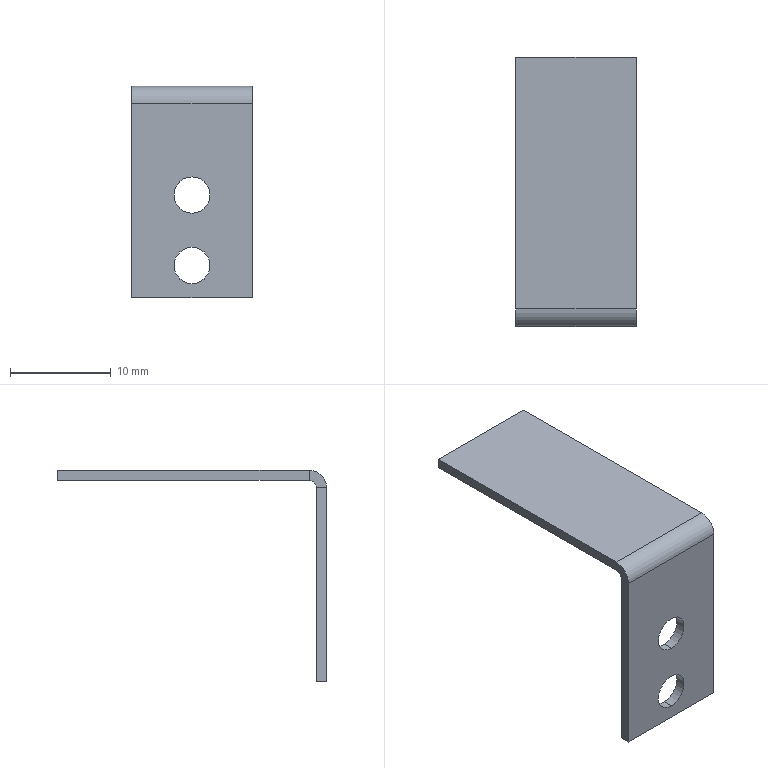Part | STEP file | PN_0031(Default) | 1 solid | 18 faces | box 12 x 26.737 x 21 mm | volume 534.113 mm3 | plane 12 | cylinder 6 | commonest cylinder face diameters 3.6 x4 1.473 x1 3.473 x1
STEP:
#1=CARTESIAN_POINT('',(0.,0.,0.));
#2=DIRECTION('',(0.,0.,1.));
#3=DIRECTION('',(1.,0.,0.));
#4=AXIS2_PLACEMENT_3D('',#1,#2,#3);
#5=CARTESIAN_POINT('',(0.,-0.7366,-12.6));
#6=VERTEX_POINT('',#5);
#7=CARTESIAN_POINT('',(0.,-1.737,-12.6));
#8=VERTEX_POINT('',#7);
#9=CARTESIAN_POINT('',(0.,-1.737,-12.6));
#10=DIRECTION('',(0.,-1.,0.));
#11=VECTOR('',#10,1.);
#12=LINE('',#9,#11);
#13=CARTESIAN_POINT('',(0.,-1.737,-10.8));
#14=DIRECTION('',(0.,-1.,0.));
#15=DIRECTION('',(0.,0.,-1.));
#16=AXIS2_PLACEMENT_3D('',#13,#14,#15);
#17=CYLINDRICAL_SURFACE('',#16,1.8);
#18=CARTESIAN_POINT('',(6.283,0.));
#19=DIRECTION('',(0.,1.));
#20=VECTOR('',#19,1.);
#21=LINE('',#18,#20);
#22=(GEOMETRIC_REPRESENTATION_CONTEXT(2)PARAMETRIC_REPRESENTATION_CONTEXT()REPRESENTATION_CONTEXT('',''));
#23=DEFINITIONAL_REPRESENTATION('',(#21),#22);
#24=PCURVE('',#17,#23);
#25=CARTESIAN_POINT('',(0.,-1.737,-10.8));
#26=DIRECTION('',(0.,-1.,0.));
#27=DIRECTION('',(0.,0.,-1.));
#28=AXIS2_PLACEMENT_3D('',#25,#26,#27);
#29=CYLINDRICAL_SURFACE('',#28,1.8);
#30=CARTESIAN_POINT('',(0.,0.));
#31=DIRECTION('',(0.,1.));
#32=VECTOR('',#31,1.);
#33=LINE('',#30,#32);
#34=(GEOMETRIC_REPRESENTATION_CONTEXT(2)PARAMETRIC_REPRESENTATION_CONTEXT()REPRESENTATION_CONTEXT('',''));
#35=DEFINITIONAL_REPRESENTATION('',(#33),#34);
#36=PCURVE('',#29,#35);
#37=SURFACE_CURVE('',#12,(#24,#36),.PCURVE_S1.);
#38=EDGE_CURVE('',#6,#8,#37,.T.);
#39=ORIENTED_EDGE('',*,*,#38,.T.);
#40=CARTESIAN_POINT('',(0.,-1.737,-9.));
#41=VERTEX_POINT('',#40);
#42=CARTESIAN_POINT('',(0.,-1.737,-10.8));
#43=DIRECTION('',(0.,-1.,0.));
#44=DIRECTION('',(0.,0.,-1.));
#45=AXIS2_PLACEMENT_3D('',#42,#43,#44);
#46=CIRCLE('',#45,1.8);
#47=CARTESIAN_POINT('',(0.,0.));
#48=DIRECTION('',(1.,0.));
#49=VECTOR('',#48,1.);
#50=LINE('',#47,#49);
#51=(GEOMETRIC_REPRESENTATION_CONTEXT(2)PARAMETRIC_REPRESENTATION_CONTEXT()REPRESENTATION_CONTEXT('',''));
#52=DEFINITIONAL_REPRESENTATION('',(#50),#51);
#53=PCURVE('',#17,#52);
#54=CARTESIAN_POINT('',(0.,-1.737,0.));
#55=DIRECTION('',(0.,1.,0.));
#56=DIRECTION('',(0.,0.,1.));
#57=AXIS2_PLACEMENT_3D('',#54,#55,#56);
#58=PLANE('',#57);
#59=CARTESIAN_POINT('',(-12.6,0.));
#60=CARTESIAN_POINT('',(-12.6,3.118));
#61=CARTESIAN_POINT('',(-9.9,1.559));
#62=CARTESIAN_POINT('',(-7.2,0.));
#63=CARTESIAN_POINT('',(-9.9,-1.559));
#64=CARTESIAN_POINT('',(-12.6,-3.118));
#65=CARTESIAN_POINT('',(-12.6,0.));
#66=(BOUNDED_CURVE()B_SPLINE_CURVE(2,(#59,#60,#61,#62,#63,#64,#65),.UNSPECIFIED.,.T.,.F.)B_SPLINE_CURVE_WITH_KNOTS((1,2,2,2,2,1),(-2.094,0.,2.094,4.189,6.283,8.378),.UNSPECIFIED.)CURVE()GEOMETRIC_REPRESENTATION_ITEM()RATIONAL_B_SPLINE_CURVE((1.,0.5,1.,0.5,1.,0.5,1.))REPRESENTATION_ITEM(''));
#67=(GEOMETRIC_REPRESENTATION_CONTEXT(2)PARAMETRIC_REPRESENTATION_CONTEXT()REPRESENTATION_CONTEXT('',''));
#68=DEFINITIONAL_REPRESENTATION('',(#66),#67);
#69=PCURVE('',#58,#68);
#70=SURFACE_CURVE('',#46,(#53,#69),.PCURVE_S1.);
#71=EDGE_CURVE('',#41,#8,#70,.T.);
#72=ORIENTED_EDGE('',*,*,#71,.F.);
#73=CARTESIAN_POINT('',(0.,-0.7366,-9.));
#74=VERTEX_POINT('',#73);
#75=CARTESIAN_POINT('',(0.,-1.737,-9.));
#76=DIRECTION('',(0.,-1.,0.));
#77=VECTOR('',#76,1.);
#78=LINE('',#75,#77);
#79=CARTESIAN_POINT('',(3.142,0.));
#80=DIRECTION('',(0.,1.));
#81=VECTOR('',#80,1.);
#82=LINE('',#79,#81);
#83=(GEOMETRIC_REPRESENTATION_CONTEXT(2)PARAMETRIC_REPRESENTATION_CONTEXT()REPRESENTATION_CONTEXT('',''));
#84=DEFINITIONAL_REPRESENTATION('',(#82),#83);
#85=PCURVE('',#17,#84);
#86=CARTESIAN_POINT('',(3.142,0.));
#87=DIRECTION('',(0.,1.));
#88=VECTOR('',#87,1.);
#89=LINE('',#86,#88);
#90=(GEOMETRIC_REPRESENTATION_CONTEXT(2)PARAMETRIC_REPRESENTATION_CONTEXT()REPRESENTATION_CONTEXT('',''));
#91=DEFINITIONAL_REPRESENTATION('',(#89),#90);
#92=PCURVE('',#29,#91);
#93=SURFACE_CURVE('',#78,(#85,#92),.PCURVE_S1.);
#94=EDGE_CURVE('',#74,#41,#93,.T.);
#95=ORIENTED_EDGE('',*,*,#94,.F.);
#96=CARTESIAN_POINT('',(0.,-0.7366,-10.8));
#97=DIRECTION('',(0.,1.,0.));
#98=DIRECTION('',(0.,0.,1.));
#99=AXIS2_PLACEMENT_3D('',#96,#97,#98);
#100=CIRCLE('',#99,1.8);
#101=CARTESIAN_POINT('',(9.425,-1.));
#102=DIRECTION('',(-1.,0.));
#103=VECTOR('',#102,1.);
#104=LINE('',#101,#103);
#105=(GEOMETRIC_REPRESENTATION_CONTEXT(2)PARAMETRIC_REPRESENTATION_CONTEXT()REPRESENTATION_CONTEXT('',''));
#106=DEFINITIONAL_REPRESENTATION('',(#104),#105);
#107=PCURVE('',#17,#106);
#108=CARTESIAN_POINT('',(0.,-0.7366,0.));
#109=DIRECTION('',(0.,1.,0.));
#110=DIRECTION('',(0.,0.,1.));
#111=AXIS2_PLACEMENT_3D('',#108,#109,#110);
#112=PLANE('',#111);
#113=CARTESIAN_POINT('',(-10.8,0.));
#114=DIRECTION('',(1.,0.));
#115=AXIS2_PLACEMENT_2D('',#113,#114);
#116=CIRCLE('',#115,1.8);
#117=(GEOMETRIC_REPRESENTATION_CONTEXT(2)PARAMETRIC_REPRESENTATION_CONTEXT()REPRESENTATION_CONTEXT('',''));
#118=DEFINITIONAL_REPRESENTATION('',(#116),#117);
#119=PCURVE('',#112,#118);
#120=SURFACE_CURVE('',#100,(#107,#119),.PCURVE_S1.);
#121=EDGE_CURVE('',#6,#74,#120,.T.);
#122=ORIENTED_EDGE('',*,*,#121,.F.);
#123=EDGE_LOOP('',(#39,#72,#95,#122));
#124=FACE_BOUND('',#123,.F.);
#125=ADVANCED_FACE('',(#124),#17,.F.);
#126=CARTESIAN_POINT('',(0.,-0.7366,-19.6));
#127=VERTEX_POINT('',#126);
#128=CARTESIAN_POINT('',(0.,-1.737,-19.6));
#129=VERTEX_POINT('',#128);
#130=CARTESIAN_POINT('',(0.,-1.737,-19.6));
#131=DIRECTION('',(0.,-1.,0.));
#132=VECTOR('',#131,1.);
#133=LINE('',#130,#132);
#134=CARTESIAN_POINT('',(0.,-1.737,-17.8));
#135=DIRECTION('',(0.,-1.,0.));
#136=DIRECTION('',(0.,0.,-1.));
#137=AXIS2_PLACEMENT_3D('',#134,#135,#136);
#138=CYLINDRICAL_SURFACE('',#137,1.8);
#139=CARTESIAN_POINT('',(6.283,0.));
#140=DIRECTION('',(0.,1.));
#141=VECTOR('',#140,1.);
#142=LINE('',#139,#141);
#143=(GEOMETRIC_REPRESENTATION_CONTEXT(2)PARAMETRIC_REPRESENTATION_CONTEXT()REPRESENTATION_CONTEXT('',''));
#144=DEFINITIONAL_REPRESENTATION('',(#142),#143);
#145=PCURVE('',#138,#144);
#146=CARTESIAN_POINT('',(0.,-1.737,-17.8));
#147=DIRECTION('',(0.,-1.,0.));
#148=DIRECTION('',(0.,0.,-1.));
#149=AXIS2_PLACEMENT_3D('',#146,#147,#148);
#150=CYLINDRICAL_SURFACE('',#149,1.8);
#151=CARTESIAN_POINT('',(0.,0.));
#152=DIRECTION('',(0.,1.));
#153=VECTOR('',#152,1.);
#154=LINE('',#151,#153);
#155=(GEOMETRIC_REPRESENTATION_CONTEXT(2)PARAMETRIC_REPRESENTATION_CONTEXT()REPRESENTATION_CONTEXT('',''));
#156=DEFINITIONAL_REPRESENTATION('',(#154),#155);
#157=PCURVE('',#150,#156);
#158=SURFACE_CURVE('',#133,(#145,#157),.PCURVE_S1.);
#159=EDGE_CURVE('',#127,#129,#158,.T.);
#160=ORIENTED_EDGE('',*,*,#159,.T.);
#161=CARTESIAN_POINT('',(0.,-1.737,-16.));
#162=VERTEX_POINT('',#161);
#163=CARTESIAN_POINT('',(0.,-1.737,-17.8));
#164=DIRECTION('',(0.,-1.,0.));
#165=DIRECTION('',(0.,0.,-1.));
#166=AXIS2_PLACEMENT_3D('',#163,#164,#165);
#167=CIRCLE('',#166,1.8);
#168=CARTESIAN_POINT('',(0.,0.));
#169=DIRECTION('',(1.,0.));
#170=VECTOR('',#169,1.);
#171=LINE('',#168,#170);
#172=(GEOMETRIC_REPRESENTATION_CONTEXT(2)PARAMETRIC_REPRESENTATION_CONTEXT()REPRESENTATION_CONTEXT('',''));
#173=DEFINITIONAL_REPRESENTATION('',(#171),#172);
#174=PCURVE('',#138,#173);
#175=CARTESIAN_POINT('',(-19.6,0.));
#176=CARTESIAN_POINT('',(-19.6,3.118));
#177=CARTESIAN_POINT('',(-16.9,1.559));
#178=CARTESIAN_POINT('',(-14.2,0.));
#179=CARTESIAN_POINT('',(-16.9,-1.559));
#180=CARTESIAN_POINT('',(-19.6,-3.118));
#181=CARTESIAN_POINT('',(-19.6,0.));
#182=(BOUNDED_CURVE()B_SPLINE_CURVE(2,(#175,#176,#177,#178,#179,#180,#181),.UNSPECIFIED.,.T.,.F.)B_SPLINE_CURVE_WITH_KNOTS((1,2,2,2,2,1),(-2.094,0.,2.094,4.189,6.283,8.378),.UNSPECIFIED.)CURVE()GEOMETRIC_REPRESENTATION_ITEM()RATIONAL_B_SPLINE_CURVE((1.,0.5,1.,0.5,1.,0.5,1.))REPRESENTATION_ITEM(''));
#183=(GEOMETRIC_REPRESENTATION_CONTEXT(2)PARAMETRIC_REPRESENTATION_CONTEXT()REPRESENTATION_CONTEXT('',''));
#184=DEFINITIONAL_REPRESENTATION('',(#182),#183);
#185=PCURVE('',#58,#184);
#186=SURFACE_CURVE('',#167,(#174,#185),.PCURVE_S1.);
#187=EDGE_CURVE('',#162,#129,#186,.T.);
#188=ORIENTED_EDGE('',*,*,#187,.F.);
#189=CARTESIAN_POINT('',(0.,-0.7366,-16.));
#190=VERTEX_POINT('',#189);
#191=CARTESIAN_POINT('',(0.,-1.737,-16.));
#192=DIRECTION('',(0.,-1.,0.));
#193=VECTOR('',#192,1.);
#194=LINE('',#191,#193);
#195=CARTESIAN_POINT('',(3.142,0.));
#196=DIRECTION('',(0.,1.));
#197=VECTOR('',#196,1.);
#198=LINE('',#195,#197);
#199=(GEOMETRIC_REPRESENTATION_CONTEXT(2)PARAMETRIC_REPRESENTATION_CONTEXT()REPRESENTATION_CONTEXT('',''));
#200=DEFINITIONAL_REPRESENTATION('',(#198),#199);
#201=PCURVE('',#138,#200);
#202=CARTESIAN_POINT('',(3.142,0.));
#203=DIRECTION('',(0.,1.));
#204=VECTOR('',#203,1.);
#205=LINE('',#202,#204);
#206=(GEOMETRIC_REPRESENTATION_CONTEXT(2)PARAMETRIC_REPRESENTATION_CONTEXT()REPRESENTATION_CONTEXT('',''));
#207=DEFINITIONAL_REPRESENTATION('',(#205),#206);
#208=PCURVE('',#150,#207);
#209=SURFACE_CURVE('',#194,(#201,#208),.PCURVE_S1.);
#210=EDGE_CURVE('',#190,#162,#209,.T.);
#211=ORIENTED_EDGE('',*,*,#210,.F.);
#212=CARTESIAN_POINT('',(0.,-0.7366,-17.8));
#213=DIRECTION('',(0.,1.,0.));
#214=DIRECTION('',(0.,0.,1.));
#215=AXIS2_PLACEMENT_3D('',#212,#213,#214);
#216=CIRCLE('',#215,1.8);
#217=CARTESIAN_POINT('',(9.425,-1.));
#218=DIRECTION('',(-1.,0.));
#219=VECTOR('',#218,1.);
#220=LINE('',#217,#219);
#221=(GEOMETRIC_REPRESENTATION_CONTEXT(2)PARAMETRIC_REPRESENTATION_CONTEXT()REPRESENTATION_CONTEXT('',''));
#222=DEFINITIONAL_REPRESENTATION('',(#220),#221);
#223=PCURVE('',#138,#222);
#224=CARTESIAN_POINT('',(-17.8,0.));
#225=DIRECTION('',(1.,0.));
#226=AXIS2_PLACEMENT_2D('',#224,#225);
#227=CIRCLE('',#226,1.8);
#228=(GEOMETRIC_REPRESENTATION_CONTEXT(2)PARAMETRIC_REPRESENTATION_CONTEXT()REPRESENTATION_CONTEXT('',''));
#229=DEFINITIONAL_REPRESENTATION('',(#227),#228);
#230=PCURVE('',#112,#229);
#231=SURFACE_CURVE('',#216,(#223,#230),.PCURVE_S1.);
#232=EDGE_CURVE('',#127,#190,#231,.T.);
#233=ORIENTED_EDGE('',*,*,#232,.F.);
#234=EDGE_LOOP('',(#160,#188,#211,#233));
#235=FACE_BOUND('',#234,.F.);
#236=ADVANCED_FACE('',(#235),#138,.F.);
#237=CARTESIAN_POINT('',(-6.,25.,0.));
#238=VERTEX_POINT('',#237);
#239=CARTESIAN_POINT('',(-6.,0.,0.));
#240=VERTEX_POINT('',#239);
#241=CARTESIAN_POINT('',(-6.,25.,0.));
#242=DIRECTION('',(0.,-1.,0.));
#243=VECTOR('',#242,1.);
#244=LINE('',#241,#243);
#245=CARTESIAN_POINT('',(-6.,25.,-1.));
#246=DIRECTION('',(-1.,0.,0.));
#247=DIRECTION('',(0.,-1.,0.));
#248=AXIS2_PLACEMENT_3D('',#245,#246,#247);
#249=PLANE('',#248);
#250=CARTESIAN_POINT('',(0.,1.));
#251=DIRECTION('',(1.,0.));
#252=VECTOR('',#251,1.);
#253=LINE('',#250,#252);
#254=(GEOMETRIC_REPRESENTATION_CONTEXT(2)PARAMETRIC_REPRESENTATION_CONTEXT()REPRESENTATION_CONTEXT('',''));
#255=DEFINITIONAL_REPRESENTATION('',(#253),#254);
#256=PCURVE('',#249,#255);
#257=CARTESIAN_POINT('',(0.,0.,0.));
#258=DIRECTION('',(0.,0.,1.));
#259=DIRECTION('',(1.,0.,0.));
#260=AXIS2_PLACEMENT_3D('',#257,#258,#259);
#261=PLANE('',#260);
#262=CARTESIAN_POINT('',(-6.,25.));
#263=DIRECTION('',(0.,-1.));
#264=VECTOR('',#263,1.);
#265=LINE('',#262,#264);
#266=(GEOMETRIC_REPRESENTATION_CONTEXT(2)PARAMETRIC_REPRESENTATION_CONTEXT()REPRESENTATION_CONTEXT('',''));
#267=DEFINITIONAL_REPRESENTATION('',(#265),#266);
#268=PCURVE('',#261,#267);
#269=SURFACE_CURVE('',#244,(#256,#268),.PCURVE_S1.);
#270=EDGE_CURVE('',#238,#240,#269,.T.);
#271=ORIENTED_EDGE('',*,*,#270,.F.);
#272=CARTESIAN_POINT('',(-6.,25.,-1.));
#273=VERTEX_POINT('',#272);
#274=CARTESIAN_POINT('',(-6.,25.,-1.));
#275=DIRECTION('',(0.,0.,1.));
#276=VECTOR('',#275,1.);
#277=LINE('',#274,#276);
#278=CARTESIAN_POINT('',(0.,0.));
#279=DIRECTION('',(0.,1.));
#280=VECTOR('',#279,1.);
#281=LINE('',#278,#280);
#282=(GEOMETRIC_REPRESENTATION_CONTEXT(2)PARAMETRIC_REPRESENTATION_CONTEXT()REPRESENTATION_CONTEXT('',''));
#283=DEFINITIONAL_REPRESENTATION('',(#281),#282);
#284=PCURVE('',#249,#283);
#285=CARTESIAN_POINT('',(-6.,25.,-1.));
#286=DIRECTION('',(0.,1.,0.));
#287=DIRECTION('',(0.,0.,1.));
#288=AXIS2_PLACEMENT_3D('',#285,#286,#287);
#289=PLANE('',#288);
#290=CARTESIAN_POINT('',(0.,0.));
#291=DIRECTION('',(1.,0.));
#292=VECTOR('',#291,1.);
#293=LINE('',#290,#292);
#294=(GEOMETRIC_REPRESENTATION_CONTEXT(2)PARAMETRIC_REPRESENTATION_CONTEXT()REPRESENTATION_CONTEXT('',''));
#295=DEFINITIONAL_REPRESENTATION('',(#293),#294);
#296=PCURVE('',#289,#295);
#297=SURFACE_CURVE('',#277,(#284,#296),.PCURVE_S1.);
#298=EDGE_CURVE('',#273,#238,#297,.T.);
#299=ORIENTED_EDGE('',*,*,#298,.F.);
#300=CARTESIAN_POINT('',(-6.,0.,-1.));
#301=VERTEX_POINT('',#300);
#302=CARTESIAN_POINT('',(-6.,25.,-1.));
#303=DIRECTION('',(0.,-1.,0.));
#304=VECTOR('',#303,1.);
#305=LINE('',#302,#304);
#306=CARTESIAN_POINT('',(0.,0.));
#307=DIRECTION('',(1.,0.));
#308=VECTOR('',#307,1.);
#309=LINE('',#306,#308);
#310=(GEOMETRIC_REPRESENTATION_CONTEXT(2)PARAMETRIC_REPRESENTATION_CONTEXT()REPRESENTATION_CONTEXT('',''));
#311=DEFINITIONAL_REPRESENTATION('',(#309),#310);
#312=PCURVE('',#249,#311);
#313=CARTESIAN_POINT('',(0.,0.,-1.));
#314=DIRECTION('',(0.,0.,1.));
#315=DIRECTION('',(1.,0.,0.));
#316=AXIS2_PLACEMENT_3D('',#313,#314,#315);
#317=PLANE('',#316);
#318=CARTESIAN_POINT('',(-6.,25.));
#319=DIRECTION('',(0.,-1.));
#320=VECTOR('',#319,1.);
#321=LINE('',#318,#320);
#322=(GEOMETRIC_REPRESENTATION_CONTEXT(2)PARAMETRIC_REPRESENTATION_CONTEXT()REPRESENTATION_CONTEXT('',''));
#323=DEFINITIONAL_REPRESENTATION('',(#321),#322);
#324=PCURVE('',#317,#323);
#325=SURFACE_CURVE('',#305,(#312,#324),.PCURVE_S1.);
#326=EDGE_CURVE('',#273,#301,#325,.T.);
#327=ORIENTED_EDGE('',*,*,#326,.T.);
#328=CARTESIAN_POINT('',(-6.,0.,-1.));
#329=DIRECTION('',(0.,0.,1.));
#330=VECTOR('',#329,1.);
#331=LINE('',#328,#330);
#332=CARTESIAN_POINT('',(25.,0.));
#333=DIRECTION('',(0.,1.));
#334=VECTOR('',#333,1.);
#335=LINE('',#332,#334);
#336=(GEOMETRIC_REPRESENTATION_CONTEXT(2)PARAMETRIC_REPRESENTATION_CONTEXT()REPRESENTATION_CONTEXT('',''));
#337=DEFINITIONAL_REPRESENTATION('',(#335),#336);
#338=PCURVE('',#249,#337);
#339=CARTESIAN_POINT('',(-6.,0.,-1.737));
#340=DIRECTION('',(1.,0.,0.));
#341=DIRECTION('',(0.,1.,0.));
#342=AXIS2_PLACEMENT_3D('',#339,#340,#341);
#343=PLANE('',#342);
#344=CARTESIAN_POINT('',(0.,0.7366));
#345=DIRECTION('',(0.,1.));
#346=VECTOR('',#345,1.);
#347=LINE('',#344,#346);
#348=(GEOMETRIC_REPRESENTATION_CONTEXT(2)PARAMETRIC_REPRESENTATION_CONTEXT()REPRESENTATION_CONTEXT('',''));
#349=DEFINITIONAL_REPRESENTATION('',(#347),#348);
#350=PCURVE('',#343,#349);
#351=SURFACE_CURVE('',#331,(#338,#350),.PCURVE_S1.);
#352=EDGE_CURVE('',#301,#240,#351,.T.);
#353=ORIENTED_EDGE('',*,*,#352,.T.);
#354=EDGE_LOOP('',(#271,#299,#327,#353));
#355=FACE_BOUND('',#354,.T.);
#356=ADVANCED_FACE('',(#355),#249,.T.);
#357=CARTESIAN_POINT('',(6.,25.,0.));
#358=VERTEX_POINT('',#357);
#359=CARTESIAN_POINT('',(-6.,25.,0.));
#360=DIRECTION('',(-1.,0.,0.));
#361=VECTOR('',#360,1.);
#362=LINE('',#359,#361);
#363=CARTESIAN_POINT('',(1.,0.));
#364=DIRECTION('',(0.,-1.));
#365=VECTOR('',#364,1.);
#366=LINE('',#363,#365);
#367=(GEOMETRIC_REPRESENTATION_CONTEXT(2)PARAMETRIC_REPRESENTATION_CONTEXT()REPRESENTATION_CONTEXT('',''));
#368=DEFINITIONAL_REPRESENTATION('',(#366),#367);
#369=PCURVE('',#289,#368);
#370=CARTESIAN_POINT('',(-6.,25.));
#371=DIRECTION('',(-1.,0.));
#372=VECTOR('',#371,1.);
#373=LINE('',#370,#372);
#374=(GEOMETRIC_REPRESENTATION_CONTEXT(2)PARAMETRIC_REPRESENTATION_CONTEXT()REPRESENTATION_CONTEXT('',''));
#375=DEFINITIONAL_REPRESENTATION('',(#373),#374);
#376=PCURVE('',#261,#375);
#377=SURFACE_CURVE('',#362,(#369,#376),.PCURVE_S1.);
#378=EDGE_CURVE('',#358,#238,#377,.T.);
#379=ORIENTED_EDGE('',*,*,#378,.F.);
#380=CARTESIAN_POINT('',(6.,25.,-1.));
#381=VERTEX_POINT('',#380);
#382=CARTESIAN_POINT('',(6.,25.,-1.));
#383=DIRECTION('',(0.,0.,1.));
#384=VECTOR('',#383,1.);
#385=LINE('',#382,#384);
#386=CARTESIAN_POINT('',(0.,12.));
#387=DIRECTION('',(1.,0.));
#388=VECTOR('',#387,1.);
#389=LINE('',#386,#388);
#390=(GEOMETRIC_REPRESENTATION_CONTEXT(2)PARAMETRIC_REPRESENTATION_CONTEXT()REPRESENTATION_CONTEXT('',''));
#391=DEFINITIONAL_REPRESENTATION('',(#389),#390);
#392=PCURVE('',#289,#391);
#393=CARTESIAN_POINT('',(6.,25.,-1.));
#394=DIRECTION('',(1.,0.,0.));
#395=DIRECTION('',(0.,1.,0.));
#396=AXIS2_PLACEMENT_3D('',#393,#394,#395);
#397=PLANE('',#396);
#398=CARTESIAN_POINT('',(0.,0.));
#399=DIRECTION('',(0.,1.));
#400=VECTOR('',#399,1.);
#401=LINE('',#398,#400);
#402=(GEOMETRIC_REPRESENTATION_CONTEXT(2)PARAMETRIC_REPRESENTATION_CONTEXT()REPRESENTATION_CONTEXT('',''));
#403=DEFINITIONAL_REPRESENTATION('',(#401),#402);
#404=PCURVE('',#397,#403);
#405=SURFACE_CURVE('',#385,(#392,#404),.PCURVE_S1.);
#406=EDGE_CURVE('',#381,#358,#405,.T.);
#407=ORIENTED_EDGE('',*,*,#406,.F.);
#408=CARTESIAN_POINT('',(-6.,25.,-1.));
#409=DIRECTION('',(-1.,0.,0.));
#410=VECTOR('',#409,1.);
#411=LINE('',#408,#410);
#412=CARTESIAN_POINT('',(0.,0.));
#413=DIRECTION('',(0.,-1.));
#414=VECTOR('',#413,1.);
#415=LINE('',#412,#414);
#416=(GEOMETRIC_REPRESENTATION_CONTEXT(2)PARAMETRIC_REPRESENTATION_CONTEXT()REPRESENTATION_CONTEXT('',''));
#417=DEFINITIONAL_REPRESENTATION('',(#415),#416);
#418=PCURVE('',#289,#417);
#419=CARTESIAN_POINT('',(-6.,25.));
#420=DIRECTION('',(-1.,0.));
#421=VECTOR('',#420,1.);
#422=LINE('',#419,#421);
#423=(GEOMETRIC_REPRESENTATION_CONTEXT(2)PARAMETRIC_REPRESENTATION_CONTEXT()REPRESENTATION_CONTEXT('',''));
#424=DEFINITIONAL_REPRESENTATION('',(#422),#423);
#425=PCURVE('',#317,#424);
#426=SURFACE_CURVE('',#411,(#418,#425),.PCURVE_S1.);
#427=EDGE_CURVE('',#381,#273,#426,.T.);
#428=ORIENTED_EDGE('',*,*,#427,.T.);
#429=ORIENTED_EDGE('',*,*,#298,.T.);
#430=EDGE_LOOP('',(#379,#407,#428,#429));
#431=FACE_BOUND('',#430,.T.);
#432=ADVANCED_FACE('',(#431),#289,.T.);
#433=CARTESIAN_POINT('',(6.,0.,0.));
#434=VERTEX_POINT('',#433);
#435=CARTESIAN_POINT('',(6.,25.,0.));
#436=DIRECTION('',(0.,1.,0.));
#437=VECTOR('',#436,1.);
#438=LINE('',#435,#437);
#439=CARTESIAN_POINT('',(0.,1.));
#440=DIRECTION('',(1.,0.));
#441=VECTOR('',#440,1.);
#442=LINE('',#439,#441);
#443=(GEOMETRIC_REPRESENTATION_CONTEXT(2)PARAMETRIC_REPRESENTATION_CONTEXT()REPRESENTATION_CONTEXT('',''));
#444=DEFINITIONAL_REPRESENTATION('',(#442),#443);
#445=PCURVE('',#397,#444);
#446=CARTESIAN_POINT('',(6.,25.));
#447=DIRECTION('',(0.,1.));
#448=VECTOR('',#447,1.);
#449=LINE('',#446,#448);
#450=(GEOMETRIC_REPRESENTATION_CONTEXT(2)PARAMETRIC_REPRESENTATION_CONTEXT()REPRESENTATION_CONTEXT('',''));
#451=DEFINITIONAL_REPRESENTATION('',(#449),#450);
#452=PCURVE('',#261,#451);
#453=SURFACE_CURVE('',#438,(#445,#452),.PCURVE_S1.);
#454=EDGE_CURVE('',#434,#358,#453,.T.);
#455=ORIENTED_EDGE('',*,*,#454,.F.);
#456=CARTESIAN_POINT('',(6.,0.,-1.));
#457=VERTEX_POINT('',#456);
#458=CARTESIAN_POINT('',(6.,0.,-1.));
#459=DIRECTION('',(0.,0.,1.));
#460=VECTOR('',#459,1.);
#461=LINE('',#458,#460);
#462=CARTESIAN_POINT('',(-25.,0.));
#463=DIRECTION('',(0.,1.));
#464=VECTOR('',#463,1.);
#465=LINE('',#462,#464);
#466=(GEOMETRIC_REPRESENTATION_CONTEXT(2)PARAMETRIC_REPRESENTATION_CONTEXT()REPRESENTATION_CONTEXT('',''));
#467=DEFINITIONAL_REPRESENTATION('',(#465),#466);
#468=PCURVE('',#397,#467);
#469=CARTESIAN_POINT('',(6.,0.,-1.737));
#470=DIRECTION('',(1.,0.,0.));
#471=DIRECTION('',(0.,1.,0.));
#472=AXIS2_PLACEMENT_3D('',#469,#470,#471);
#473=PLANE('',#472);
#474=CARTESIAN_POINT('',(0.,0.7366));
#475=DIRECTION('',(0.,1.));
#476=VECTOR('',#475,1.);
#477=LINE('',#474,#476);
#478=(GEOMETRIC_REPRESENTATION_CONTEXT(2)PARAMETRIC_REPRESENTATION_CONTEXT()REPRESENTATION_CONTEXT('',''));
#479=DEFINITIONAL_REPRESENTATION('',(#477),#478);
#480=PCURVE('',#473,#479);
#481=SURFACE_CURVE('',#461,(#468,#480),.PCURVE_S1.);
#482=EDGE_CURVE('',#457,#434,#481,.T.);
#483=ORIENTED_EDGE('',*,*,#482,.F.);
#484=CARTESIAN_POINT('',(6.,25.,-1.));
#485=DIRECTION('',(0.,1.,0.));
#486=VECTOR('',#485,1.);
#487=LINE('',#484,#486);
#488=CARTESIAN_POINT('',(0.,0.));
#489=DIRECTION('',(1.,0.));
#490=VECTOR('',#489,1.);
#491=LINE('',#488,#490);
#492=(GEOMETRIC_REPRESENTATION_CONTEXT(2)PARAMETRIC_REPRESENTATION_CONTEXT()REPRESENTATION_CONTEXT('',''));
#493=DEFINITIONAL_REPRESENTATION('',(#491),#492);
#494=PCURVE('',#397,#493);
#495=CARTESIAN_POINT('',(6.,25.));
#496=DIRECTION('',(0.,1.));
#497=VECTOR('',#496,1.);
#498=LINE('',#495,#497);
#499=(GEOMETRIC_REPRESENTATION_CONTEXT(2)PARAMETRIC_REPRESENTATION_CONTEXT()REPRESENTATION_CONTEXT('',''));
#500=DEFINITIONAL_REPRESENTATION('',(#498),#499);
#501=PCURVE('',#317,#500);
#502=SURFACE_CURVE('',#487,(#494,#501),.PCURVE_S1.);
#503=EDGE_CURVE('',#457,#381,#502,.T.);
#504=ORIENTED_EDGE('',*,*,#503,.T.);
#505=ORIENTED_EDGE('',*,*,#406,.T.);
#506=EDGE_LOOP('',(#455,#483,#504,#505));
#507=FACE_BOUND('',#506,.T.);
#508=ADVANCED_FACE('',(#507),#397,.T.);
#509=ORIENTED_EDGE('',*,*,#326,.F.);
#510=ORIENTED_EDGE('',*,*,#427,.F.);
#511=ORIENTED_EDGE('',*,*,#503,.F.);
#512=CARTESIAN_POINT('',(-6.,0.,-1.));
#513=DIRECTION('',(1.,0.,0.));
#514=VECTOR('',#513,1.);
#515=LINE('',#512,#514);
#516=CARTESIAN_POINT('',(-6.,0.));
#517=DIRECTION('',(1.,0.));
#518=VECTOR('',#517,1.);
#519=LINE('',#516,#518);
#520=(GEOMETRIC_REPRESENTATION_CONTEXT(2)PARAMETRIC_REPRESENTATION_CONTEXT()REPRESENTATION_CONTEXT('',''));
#521=DEFINITIONAL_REPRESENTATION('',(#519),#520);
#522=PCURVE('',#317,#521);
#523=CARTESIAN_POINT('',(-6.,0.,-1.737));
#524=DIRECTION('',(-1.,0.,0.));
#525=DIRECTION('',(0.,-1.,0.));
#526=AXIS2_PLACEMENT_3D('',#523,#524,#525);
#527=CYLINDRICAL_SURFACE('',#526,0.7366);
#528=CARTESIAN_POINT('',(1.571,0.));
#529=DIRECTION('',(0.,-1.));
#530=VECTOR('',#529,1.);
#531=LINE('',#528,#530);
#532=(GEOMETRIC_REPRESENTATION_CONTEXT(2)PARAMETRIC_REPRESENTATION_CONTEXT()REPRESENTATION_CONTEXT('',''));
#533=DEFINITIONAL_REPRESENTATION('',(#531),#532);
#534=PCURVE('',#527,#533);
#535=SURFACE_CURVE('',#515,(#522,#534),.PCURVE_S1.);
#536=EDGE_CURVE('',#301,#457,#535,.T.);
#537=ORIENTED_EDGE('',*,*,#536,.F.);
#538=EDGE_LOOP('',(#509,#510,#511,#537));
#539=FACE_BOUND('',#538,.T.);
#540=ADVANCED_FACE('',(#539),#317,.F.);
#541=ORIENTED_EDGE('',*,*,#270,.T.);
#542=CARTESIAN_POINT('',(-6.,0.,0.));
#543=DIRECTION('',(1.,0.,0.));
#544=VECTOR('',#543,1.);
#545=LINE('',#542,#544);
#546=CARTESIAN_POINT('',(-6.,0.));
#547=DIRECTION('',(1.,0.));
#548=VECTOR('',#547,1.);
#549=LINE('',#546,#548);
#550=(GEOMETRIC_REPRESENTATION_CONTEXT(2)PARAMETRIC_REPRESENTATION_CONTEXT()REPRESENTATION_CONTEXT('',''));
#551=DEFINITIONAL_REPRESENTATION('',(#549),#550);
#552=PCURVE('',#261,#551);
#553=CARTESIAN_POINT('',(-6.,0.,-1.737));
#554=DIRECTION('',(-1.,0.,0.));
#555=DIRECTION('',(0.,-1.,0.));
#556=AXIS2_PLACEMENT_3D('',#553,#554,#555);
#557=CYLINDRICAL_SURFACE('',#556,1.737);
#558=CARTESIAN_POINT('',(1.571,0.));
#559=DIRECTION('',(0.,-1.));
#560=VECTOR('',#559,1.);
#561=LINE('',#558,#560);
#562=(GEOMETRIC_REPRESENTATION_CONTEXT(2)PARAMETRIC_REPRESENTATION_CONTEXT()REPRESENTATION_CONTEXT('',''));
#563=DEFINITIONAL_REPRESENTATION('',(#561),#562);
#564=PCURVE('',#557,#563);
#565=SURFACE_CURVE('',#545,(#552,#564),.PCURVE_S1.);
#566=EDGE_CURVE('',#240,#434,#565,.T.);
#567=ORIENTED_EDGE('',*,*,#566,.T.);
#568=ORIENTED_EDGE('',*,*,#454,.T.);
#569=ORIENTED_EDGE('',*,*,#378,.T.);
#570=EDGE_LOOP('',(#541,#567,#568,#569));
#571=FACE_BOUND('',#570,.T.);
#572=ADVANCED_FACE('',(#571),#261,.T.);
#573=CARTESIAN_POINT('',(6.,-0.7366,-1.737));
#574=VERTEX_POINT('',#573);
#575=CARTESIAN_POINT('',(6.,-1.737,-1.737));
#576=VERTEX_POINT('',#575);
#577=CARTESIAN_POINT('',(6.,-1.737,-1.737));
#578=DIRECTION('',(0.,-1.,0.));
#579=VECTOR('',#578,1.);
#580=LINE('',#577,#579);
#581=CARTESIAN_POINT('',(-1.737,0.));
#582=DIRECTION('',(-1.,0.));
#583=VECTOR('',#582,1.);
#584=LINE('',#581,#583);
#585=(GEOMETRIC_REPRESENTATION_CONTEXT(2)PARAMETRIC_REPRESENTATION_CONTEXT()REPRESENTATION_CONTEXT('',''));
#586=DEFINITIONAL_REPRESENTATION('',(#584),#585);
#587=PCURVE('',#473,#586);
#588=CARTESIAN_POINT('',(6.,-1.737,-1.));
#589=DIRECTION('',(-1.,0.,0.));
#590=DIRECTION('',(0.,0.,1.));
#591=AXIS2_PLACEMENT_3D('',#588,#589,#590);
#592=PLANE('',#591);
#593=CARTESIAN_POINT('',(-0.7366,0.));
#594=DIRECTION('',(0.,-1.));
#595=VECTOR('',#594,1.);
#596=LINE('',#593,#595);
#597=(GEOMETRIC_REPRESENTATION_CONTEXT(2)PARAMETRIC_REPRESENTATION_CONTEXT()REPRESENTATION_CONTEXT('',''));
#598=DEFINITIONAL_REPRESENTATION('',(#596),#597);
#599=PCURVE('',#592,#598);
#600=SURFACE_CURVE('',#580,(#587,#599),.PCURVE_S1.);
#601=EDGE_CURVE('',#574,#576,#600,.T.);
#602=ORIENTED_EDGE('',*,*,#601,.F.);
#603=CARTESIAN_POINT('',(6.,0.,-1.737));
#604=DIRECTION('',(1.,0.,0.));
#605=DIRECTION('',(0.,-1.,0.));
#606=AXIS2_PLACEMENT_3D('',#603,#604,#605);
#607=CIRCLE('',#606,0.7366);
#608=CARTESIAN_POINT('',(0.,0.));
#609=DIRECTION('',(-1.,0.));
#610=AXIS2_PLACEMENT_2D('',#608,#609);
#611=CIRCLE('',#610,0.7366);
#612=(GEOMETRIC_REPRESENTATION_CONTEXT(2)PARAMETRIC_REPRESENTATION_CONTEXT()REPRESENTATION_CONTEXT('',''));
#613=DEFINITIONAL_REPRESENTATION('',(#611),#612);
#614=PCURVE('',#473,#613);
#615=CARTESIAN_POINT('',(6.283,-12.));
#616=DIRECTION('',(-1.,0.));
#617=VECTOR('',#616,1.);
#618=LINE('',#615,#617);
#619=(GEOMETRIC_REPRESENTATION_CONTEXT(2)PARAMETRIC_REPRESENTATION_CONTEXT()REPRESENTATION_CONTEXT('',''));
#620=DEFINITIONAL_REPRESENTATION('',(#618),#619);
#621=PCURVE('',#527,#620);
#622=SURFACE_CURVE('',#607,(#614,#621),.PCURVE_S1.);
#623=EDGE_CURVE('',#457,#574,#622,.T.);
#624=ORIENTED_EDGE('',*,*,#623,.F.);
#625=ORIENTED_EDGE('',*,*,#482,.T.);
#626=CARTESIAN_POINT('',(6.,0.,-1.737));
#627=DIRECTION('',(1.,0.,0.));
#628=DIRECTION('',(0.,-1.,0.));
#629=AXIS2_PLACEMENT_3D('',#626,#627,#628);
#630=CIRCLE('',#629,1.737);
#631=CARTESIAN_POINT('',(0.,0.));
#632=DIRECTION('',(-1.,0.));
#633=AXIS2_PLACEMENT_2D('',#631,#632);
#634=CIRCLE('',#633,1.737);
#635=(GEOMETRIC_REPRESENTATION_CONTEXT(2)PARAMETRIC_REPRESENTATION_CONTEXT()REPRESENTATION_CONTEXT('',''));
#636=DEFINITIONAL_REPRESENTATION('',(#634),#635);
#637=PCURVE('',#473,#636);
#638=CARTESIAN_POINT('',(6.283,-12.));
#639=DIRECTION('',(-1.,0.));
#640=VECTOR('',#639,1.);
#641=LINE('',#638,#640);
#642=(GEOMETRIC_REPRESENTATION_CONTEXT(2)PARAMETRIC_REPRESENTATION_CONTEXT()REPRESENTATION_CONTEXT('',''));
#643=DEFINITIONAL_REPRESENTATION('',(#641),#642);
#644=PCURVE('',#557,#643);
#645=SURFACE_CURVE('',#630,(#637,#644),.PCURVE_S1.);
#646=EDGE_CURVE('',#434,#576,#645,.T.);
#647=ORIENTED_EDGE('',*,*,#646,.T.);
#648=EDGE_LOOP('',(#602,#624,#625,#647));
#649=FACE_BOUND('',#648,.T.);
#650=ADVANCED_FACE('',(#649),#473,.T.);
#651=CARTESIAN_POINT('',(-6.,-0.7366,-1.737));
#652=VERTEX_POINT('',#651);
#653=CARTESIAN_POINT('',(-6.,0.,-1.737));
#654=DIRECTION('',(-1.,0.,0.));
#655=DIRECTION('',(0.,-1.,0.));
#656=AXIS2_PLACEMENT_3D('',#653,#654,#655);
#657=CIRCLE('',#656,0.7366);
#658=CARTESIAN_POINT('',(-0.7366,0.));
#659=CARTESIAN_POINT('',(-0.7366,1.276));
#660=CARTESIAN_POINT('',(0.3683,0.6379));
#661=CARTESIAN_POINT('',(1.473,0.));
#662=CARTESIAN_POINT('',(0.3683,-0.6379));
#663=CARTESIAN_POINT('',(-0.7366,-1.276));
#664=CARTESIAN_POINT('',(-0.7366,0.));
#665=(BOUNDED_CURVE()B_SPLINE_CURVE(2,(#658,#659,#660,#661,#662,#663,#664),.UNSPECIFIED.,.T.,.F.)B_SPLINE_CURVE_WITH_KNOTS((1,2,2,2,2,1),(-2.094,0.,2.094,4.189,6.283,8.378),.UNSPECIFIED.)CURVE()GEOMETRIC_REPRESENTATION_ITEM()RATIONAL_B_SPLINE_CURVE((1.,0.5,1.,0.5,1.,0.5,1.))REPRESENTATION_ITEM(''));
#666=(GEOMETRIC_REPRESENTATION_CONTEXT(2)PARAMETRIC_REPRESENTATION_CONTEXT()REPRESENTATION_CONTEXT('',''));
#667=DEFINITIONAL_REPRESENTATION('',(#665),#666);
#668=PCURVE('',#343,#667);
#669=CARTESIAN_POINT('',(0.,0.));
#670=DIRECTION('',(1.,0.));
#671=VECTOR('',#670,1.);
#672=LINE('',#669,#671);
#673=(GEOMETRIC_REPRESENTATION_CONTEXT(2)PARAMETRIC_REPRESENTATION_CONTEXT()REPRESENTATION_CONTEXT('',''));
#674=DEFINITIONAL_REPRESENTATION('',(#672),#673);
#675=PCURVE('',#527,#674);
#676=SURFACE_CURVE('',#657,(#668,#675),.PCURVE_S1.);
#677=EDGE_CURVE('',#652,#301,#676,.T.);
#678=ORIENTED_EDGE('',*,*,#677,.F.);
#679=CARTESIAN_POINT('',(-6.,-1.737,-1.737));
#680=VERTEX_POINT('',#679);
#681=CARTESIAN_POINT('',(-6.,-0.7366,-1.737));
#682=DIRECTION('',(0.,-1.,0.));
#683=VECTOR('',#682,1.);
#684=LINE('',#681,#683);
#685=CARTESIAN_POINT('',(-0.7366,0.));
#686=DIRECTION('',(-1.,0.));
#687=VECTOR('',#686,1.);
#688=LINE('',#685,#687);
#689=(GEOMETRIC_REPRESENTATION_CONTEXT(2)PARAMETRIC_REPRESENTATION_CONTEXT()REPRESENTATION_CONTEXT('',''));
#690=DEFINITIONAL_REPRESENTATION('',(#688),#689);
#691=PCURVE('',#343,#690);
#692=CARTESIAN_POINT('',(-6.,-1.737,-21.));
#693=DIRECTION('',(1.,0.,0.));
#694=DIRECTION('',(0.,0.,-1.));
#695=AXIS2_PLACEMENT_3D('',#692,#693,#694);
#696=PLANE('',#695);
#697=CARTESIAN_POINT('',(-19.263,1.));
#698=DIRECTION('',(0.,-1.));
#699=VECTOR('',#698,1.);
#700=LINE('',#697,#699);
#701=(GEOMETRIC_REPRESENTATION_CONTEXT(2)PARAMETRIC_REPRESENTATION_CONTEXT()REPRESENTATION_CONTEXT('',''));
#702=DEFINITIONAL_REPRESENTATION('',(#700),#701);
#703=PCURVE('',#696,#702);
#704=SURFACE_CURVE('',#684,(#691,#703),.PCURVE_S1.);
#705=EDGE_CURVE('',#652,#680,#704,.T.);
#706=ORIENTED_EDGE('',*,*,#705,.T.);
#707=CARTESIAN_POINT('',(-6.,0.,-1.737));
#708=DIRECTION('',(-1.,0.,0.));
#709=DIRECTION('',(0.,-1.,0.));
#710=AXIS2_PLACEMENT_3D('',#707,#708,#709);
#711=CIRCLE('',#710,1.737);
#712=CARTESIAN_POINT('',(-1.737,0.));
#713=CARTESIAN_POINT('',(-1.737,3.008));
#714=CARTESIAN_POINT('',(0.8683,1.504));
#715=CARTESIAN_POINT('',(3.473,0.));
#716=CARTESIAN_POINT('',(0.8683,-1.504));
#717=CARTESIAN_POINT('',(-1.737,-3.008));
#718=CARTESIAN_POINT('',(-1.737,0.));
#719=(BOUNDED_CURVE()B_SPLINE_CURVE(2,(#712,#713,#714,#715,#716,#717,#718),.UNSPECIFIED.,.T.,.F.)B_SPLINE_CURVE_WITH_KNOTS((1,2,2,2,2,1),(-2.094,0.,2.094,4.189,6.283,8.378),.UNSPECIFIED.)CURVE()GEOMETRIC_REPRESENTATION_ITEM()RATIONAL_B_SPLINE_CURVE((1.,0.5,1.,0.5,1.,0.5,1.))REPRESENTATION_ITEM(''));
#720=(GEOMETRIC_REPRESENTATION_CONTEXT(2)PARAMETRIC_REPRESENTATION_CONTEXT()REPRESENTATION_CONTEXT('',''));
#721=DEFINITIONAL_REPRESENTATION('',(#719),#720);
#722=PCURVE('',#343,#721);
#723=CARTESIAN_POINT('',(0.,0.));
#724=DIRECTION('',(1.,0.));
#725=VECTOR('',#724,1.);
#726=LINE('',#723,#725);
#727=(GEOMETRIC_REPRESENTATION_CONTEXT(2)PARAMETRIC_REPRESENTATION_CONTEXT()REPRESENTATION_CONTEXT('',''));
#728=DEFINITIONAL_REPRESENTATION('',(#726),#727);
#729=PCURVE('',#557,#728);
#730=SURFACE_CURVE('',#711,(#722,#729),.PCURVE_S1.);
#731=EDGE_CURVE('',#680,#240,#730,.T.);
#732=ORIENTED_EDGE('',*,*,#731,.T.);
#733=ORIENTED_EDGE('',*,*,#352,.F.);
#734=EDGE_LOOP('',(#678,#706,#732,#733));
#735=FACE_BOUND('',#734,.T.);
#736=ADVANCED_FACE('',(#735),#343,.F.);
#737=ORIENTED_EDGE('',*,*,#566,.F.);
#738=ORIENTED_EDGE('',*,*,#731,.F.);
#739=CARTESIAN_POINT('',(6.,-1.737,-1.737));
#740=DIRECTION('',(1.,0.,0.));
#741=VECTOR('',#740,1.);
#742=LINE('',#739,#741);
#743=CARTESIAN_POINT('',(0.,-12.));
#744=DIRECTION('',(0.,-1.));
#745=VECTOR('',#744,1.);
#746=LINE('',#743,#745);
#747=(GEOMETRIC_REPRESENTATION_CONTEXT(2)PARAMETRIC_REPRESENTATION_CONTEXT()REPRESENTATION_CONTEXT('',''));
#748=DEFINITIONAL_REPRESENTATION('',(#746),#747);
#749=PCURVE('',#557,#748);
#750=CARTESIAN_POINT('',(-1.737,6.));
#751=DIRECTION('',(0.,1.));
#752=VECTOR('',#751,1.);
#753=LINE('',#750,#752);
#754=(GEOMETRIC_REPRESENTATION_CONTEXT(2)PARAMETRIC_REPRESENTATION_CONTEXT()REPRESENTATION_CONTEXT('',''));
#755=DEFINITIONAL_REPRESENTATION('',(#753),#754);
#756=PCURVE('',#58,#755);
#757=SURFACE_CURVE('',#742,(#749,#756),.PCURVE_S1.);
#758=EDGE_CURVE('',#680,#576,#757,.T.);
#759=ORIENTED_EDGE('',*,*,#758,.T.);
#760=ORIENTED_EDGE('',*,*,#646,.F.);
#761=EDGE_LOOP('',(#737,#738,#759,#760));
#762=FACE_BOUND('',#761,.T.);
#763=ADVANCED_FACE('',(#762),#557,.T.);
#764=ORIENTED_EDGE('',*,*,#677,.F.);
#765=CARTESIAN_POINT('',(6.,-0.7366,-1.737));
#766=DIRECTION('',(-1.,0.,0.));
#767=VECTOR('',#766,1.);
#768=LINE('',#765,#767);
#769=CARTESIAN_POINT('',(0.,-12.));
#770=DIRECTION('',(0.,1.));
#771=VECTOR('',#770,1.);
#772=LINE('',#769,#771);
#773=(GEOMETRIC_REPRESENTATION_CONTEXT(2)PARAMETRIC_REPRESENTATION_CONTEXT()REPRESENTATION_CONTEXT('',''));
#774=DEFINITIONAL_REPRESENTATION('',(#772),#773);
#775=PCURVE('',#527,#774);
#776=CARTESIAN_POINT('',(-1.737,6.));
#777=DIRECTION('',(0.,-1.));
#778=VECTOR('',#777,1.);
#779=LINE('',#776,#778);
#780=(GEOMETRIC_REPRESENTATION_CONTEXT(2)PARAMETRIC_REPRESENTATION_CONTEXT()REPRESENTATION_CONTEXT('',''));
#781=DEFINITIONAL_REPRESENTATION('',(#779),#780);
#782=PCURVE('',#112,#781);
#783=SURFACE_CURVE('',#768,(#775,#782),.PCURVE_S1.);
#784=EDGE_CURVE('',#574,#652,#783,.T.);
#785=ORIENTED_EDGE('',*,*,#784,.F.);
#786=ORIENTED_EDGE('',*,*,#623,.F.);
#787=ORIENTED_EDGE('',*,*,#536,.F.);
#788=EDGE_LOOP('',(#764,#785,#786,#787));
#789=FACE_BOUND('',#788,.F.);
#790=ADVANCED_FACE('',(#789),#527,.F.);
#791=ORIENTED_EDGE('',*,*,#705,.F.);
#792=CARTESIAN_POINT('',(-6.,-0.7366,-21.));
#793=VERTEX_POINT('',#792);
#794=CARTESIAN_POINT('',(-6.,-0.7366,-21.));
#795=DIRECTION('',(0.,0.,-1.));
#796=VECTOR('',#795,1.);
#797=LINE('',#794,#796);
#798=CARTESIAN_POINT('',(0.,1.));
#799=DIRECTION('',(1.,0.));
#800=VECTOR('',#799,1.);
#801=LINE('',#798,#800);
#802=(GEOMETRIC_REPRESENTATION_CONTEXT(2)PARAMETRIC_REPRESENTATION_CONTEXT()REPRESENTATION_CONTEXT('',''));
#803=DEFINITIONAL_REPRESENTATION('',(#801),#802);
#804=PCURVE('',#696,#803);
#805=CARTESIAN_POINT('',(-21.,-6.));
#806=DIRECTION('',(-1.,0.));
#807=VECTOR('',#806,1.);
#808=LINE('',#805,#807);
#809=(GEOMETRIC_REPRESENTATION_CONTEXT(2)PARAMETRIC_REPRESENTATION_CONTEXT()REPRESENTATION_CONTEXT('',''));
#810=DEFINITIONAL_REPRESENTATION('',(#808),#809);
#811=PCURVE('',#112,#810);
#812=SURFACE_CURVE('',#797,(#804,#811),.PCURVE_S1.);
#813=EDGE_CURVE('',#652,#793,#812,.T.);
#814=ORIENTED_EDGE('',*,*,#813,.T.);
#815=CARTESIAN_POINT('',(-6.,-1.737,-21.));
#816=VERTEX_POINT('',#815);
#817=CARTESIAN_POINT('',(-6.,-1.737,-21.));
#818=DIRECTION('',(0.,1.,0.));
#819=VECTOR('',#818,1.);
#820=LINE('',#817,#819);
#821=CARTESIAN_POINT('',(0.,0.));
#822=DIRECTION('',(0.,1.));
#823=VECTOR('',#822,1.);
#824=LINE('',#821,#823);
#825=(GEOMETRIC_REPRESENTATION_CONTEXT(2)PARAMETRIC_REPRESENTATION_CONTEXT()REPRESENTATION_CONTEXT('',''));
#826=DEFINITIONAL_REPRESENTATION('',(#824),#825);
#827=PCURVE('',#696,#826);
#828=CARTESIAN_POINT('',(6.,-1.737,-21.));
#829=DIRECTION('',(0.,0.,1.));
#830=DIRECTION('',(0.,-1.,0.));
#831=AXIS2_PLACEMENT_3D('',#828,#829,#830);
#832=PLANE('',#831);
#833=CARTESIAN_POINT('',(0.,-12.));
#834=DIRECTION('',(-1.,0.));
#835=VECTOR('',#834,1.);
#836=LINE('',#833,#835);
#837=(GEOMETRIC_REPRESENTATION_CONTEXT(2)PARAMETRIC_REPRESENTATION_CONTEXT()REPRESENTATION_CONTEXT('',''));
#838=DEFINITIONAL_REPRESENTATION('',(#836),#837);
#839=PCURVE('',#832,#838);
#840=SURFACE_CURVE('',#820,(#827,#839),.PCURVE_S1.);
#841=EDGE_CURVE('',#816,#793,#840,.T.);
#842=ORIENTED_EDGE('',*,*,#841,.F.);
#843=CARTESIAN_POINT('',(-6.,-1.737,0.));
#844=DIRECTION('',(0.,0.,-1.));
#845=VECTOR('',#844,1.);
#846=LINE('',#843,#845);
#847=CARTESIAN_POINT('',(-21.,0.));
#848=DIRECTION('',(1.,0.));
#849=VECTOR('',#848,1.);
#850=LINE('',#847,#849);
#851=(GEOMETRIC_REPRESENTATION_CONTEXT(2)PARAMETRIC_REPRESENTATION_CONTEXT()REPRESENTATION_CONTEXT('',''));
#852=DEFINITIONAL_REPRESENTATION('',(#850),#851);
#853=PCURVE('',#696,#852);
#854=CARTESIAN_POINT('',(0.,-6.));
#855=DIRECTION('',(-1.,0.));
#856=VECTOR('',#855,1.);
#857=LINE('',#854,#856);
#858=(GEOMETRIC_REPRESENTATION_CONTEXT(2)PARAMETRIC_REPRESENTATION_CONTEXT()REPRESENTATION_CONTEXT('',''));
#859=DEFINITIONAL_REPRESENTATION('',(#857),#858);
#860=PCURVE('',#58,#859);
#861=SURFACE_CURVE('',#846,(#853,#860),.PCURVE_S1.);
#862=EDGE_CURVE('',#680,#816,#861,.T.);
#863=ORIENTED_EDGE('',*,*,#862,.F.);
#864=EDGE_LOOP('',(#791,#814,#842,#863));
#865=FACE_BOUND('',#864,.T.);
#866=ADVANCED_FACE('',(#865),#696,.F.);
#867=ORIENTED_EDGE('',*,*,#601,.T.);
#868=CARTESIAN_POINT('',(6.,-1.737,-21.));
#869=VERTEX_POINT('',#868);
#870=CARTESIAN_POINT('',(6.,-1.737,0.));
#871=DIRECTION('',(0.,0.,1.));
#872=VECTOR('',#871,1.);
#873=LINE('',#870,#872);
#874=CARTESIAN_POINT('',(1.,0.));
#875=DIRECTION('',(1.,0.));
#876=VECTOR('',#875,1.);
#877=LINE('',#874,#876);
#878=(GEOMETRIC_REPRESENTATION_CONTEXT(2)PARAMETRIC_REPRESENTATION_CONTEXT()REPRESENTATION_CONTEXT('',''));
#879=DEFINITIONAL_REPRESENTATION('',(#877),#878);
#880=PCURVE('',#592,#879);
#881=CARTESIAN_POINT('',(0.,6.));
#882=DIRECTION('',(1.,0.));
#883=VECTOR('',#882,1.);
#884=LINE('',#881,#883);
#885=(GEOMETRIC_REPRESENTATION_CONTEXT(2)PARAMETRIC_REPRESENTATION_CONTEXT()REPRESENTATION_CONTEXT('',''));
#886=DEFINITIONAL_REPRESENTATION('',(#884),#885);
#887=PCURVE('',#58,#886);
#888=SURFACE_CURVE('',#873,(#880,#887),.PCURVE_S1.);
#889=EDGE_CURVE('',#869,#576,#888,.T.);
#890=ORIENTED_EDGE('',*,*,#889,.F.);
#891=CARTESIAN_POINT('',(6.,-0.7366,-21.));
#892=VERTEX_POINT('',#891);
#893=CARTESIAN_POINT('',(6.,-1.737,-21.));
#894=DIRECTION('',(0.,1.,0.));
#895=VECTOR('',#894,1.);
#896=LINE('',#893,#895);
#897=CARTESIAN_POINT('',(-20.,0.));
#898=DIRECTION('',(0.,1.));
#899=VECTOR('',#898,1.);
#900=LINE('',#897,#899);
#901=(GEOMETRIC_REPRESENTATION_CONTEXT(2)PARAMETRIC_REPRESENTATION_CONTEXT()REPRESENTATION_CONTEXT('',''));
#902=DEFINITIONAL_REPRESENTATION('',(#900),#901);
#903=PCURVE('',#592,#902);
#904=CARTESIAN_POINT('',(0.,0.));
#905=DIRECTION('',(-1.,0.));
#906=VECTOR('',#905,1.);
#907=LINE('',#904,#906);
#908=(GEOMETRIC_REPRESENTATION_CONTEXT(2)PARAMETRIC_REPRESENTATION_CONTEXT()REPRESENTATION_CONTEXT('',''));
#909=DEFINITIONAL_REPRESENTATION('',(#907),#908);
#910=PCURVE('',#832,#909);
#911=SURFACE_CURVE('',#896,(#903,#910),.PCURVE_S1.);
#912=EDGE_CURVE('',#869,#892,#911,.T.);
#913=ORIENTED_EDGE('',*,*,#912,.T.);
#914=CARTESIAN_POINT('',(6.,-0.7366,-1.));
#915=DIRECTION('',(0.,0.,1.));
#916=VECTOR('',#915,1.);
#917=LINE('',#914,#916);
#918=CARTESIAN_POINT('',(0.,1.));
#919=DIRECTION('',(1.,0.));
#920=VECTOR('',#919,1.);
#921=LINE('',#918,#920);
#922=(GEOMETRIC_REPRESENTATION_CONTEXT(2)PARAMETRIC_REPRESENTATION_CONTEXT()REPRESENTATION_CONTEXT('',''));
#923=DEFINITIONAL_REPRESENTATION('',(#921),#922);
#924=PCURVE('',#592,#923);
#925=CARTESIAN_POINT('',(-1.,6.));
#926=DIRECTION('',(1.,0.));
#927=VECTOR('',#926,1.);
#928=LINE('',#925,#927);
#929=(GEOMETRIC_REPRESENTATION_CONTEXT(2)PARAMETRIC_REPRESENTATION_CONTEXT()REPRESENTATION_CONTEXT('',''));
#930=DEFINITIONAL_REPRESENTATION('',(#928),#929);
#931=PCURVE('',#112,#930);
#932=SURFACE_CURVE('',#917,(#924,#931),.PCURVE_S1.);
#933=EDGE_CURVE('',#892,#574,#932,.T.);
#934=ORIENTED_EDGE('',*,*,#933,.T.);
#935=EDGE_LOOP('',(#867,#890,#913,#934));
#936=FACE_BOUND('',#935,.T.);
#937=ADVANCED_FACE('',(#936),#592,.F.);
#938=CARTESIAN_POINT('',(0.,-1.737,-10.8));
#939=DIRECTION('',(0.,-1.,0.));
#940=DIRECTION('',(0.,0.,-1.));
#941=AXIS2_PLACEMENT_3D('',#938,#939,#940);
#942=CIRCLE('',#941,1.8);
#943=CARTESIAN_POINT('',(-12.6,0.));
#944=CARTESIAN_POINT('',(-12.6,3.118));
#945=CARTESIAN_POINT('',(-9.9,1.559));
#946=CARTESIAN_POINT('',(-7.2,0.));
#947=CARTESIAN_POINT('',(-9.9,-1.559));
#948=CARTESIAN_POINT('',(-12.6,-3.118));
#949=CARTESIAN_POINT('',(-12.6,0.));
#950=(BOUNDED_CURVE()B_SPLINE_CURVE(2,(#943,#944,#945,#946,#947,#948,#949),.UNSPECIFIED.,.T.,.F.)B_SPLINE_CURVE_WITH_KNOTS((1,2,2,2,2,1),(-2.094,0.,2.094,4.189,6.283,8.378),.UNSPECIFIED.)CURVE()GEOMETRIC_REPRESENTATION_ITEM()RATIONAL_B_SPLINE_CURVE((1.,0.5,1.,0.5,1.,0.5,1.))REPRESENTATION_ITEM(''));
#951=(GEOMETRIC_REPRESENTATION_CONTEXT(2)PARAMETRIC_REPRESENTATION_CONTEXT()REPRESENTATION_CONTEXT('',''));
#952=DEFINITIONAL_REPRESENTATION('',(#950),#951);
#953=PCURVE('',#58,#952);
#954=CARTESIAN_POINT('',(0.,0.));
#955=DIRECTION('',(1.,0.));
#956=VECTOR('',#955,1.);
#957=LINE('',#954,#956);
#958=(GEOMETRIC_REPRESENTATION_CONTEXT(2)PARAMETRIC_REPRESENTATION_CONTEXT()REPRESENTATION_CONTEXT('',''));
#959=DEFINITIONAL_REPRESENTATION('',(#957),#958);
#960=PCURVE('',#29,#959);
#961=SURFACE_CURVE('',#942,(#953,#960),.PCURVE_S1.);
#962=EDGE_CURVE('',#8,#41,#961,.T.);
#963=ORIENTED_EDGE('',*,*,#962,.F.);
#964=ORIENTED_EDGE('',*,*,#71,.F.);
#965=EDGE_LOOP('',(#963,#964));
#966=FACE_BOUND('',#965,.T.);
#967=CARTESIAN_POINT('',(0.,-1.737,-17.8));
#968=DIRECTION('',(0.,-1.,0.));
#969=DIRECTION('',(0.,0.,-1.));
#970=AXIS2_PLACEMENT_3D('',#967,#968,#969);
#971=CIRCLE('',#970,1.8);
#972=CARTESIAN_POINT('',(-19.6,0.));
#973=CARTESIAN_POINT('',(-19.6,3.118));
#974=CARTESIAN_POINT('',(-16.9,1.559));
#975=CARTESIAN_POINT('',(-14.2,0.));
#976=CARTESIAN_POINT('',(-16.9,-1.559));
#977=CARTESIAN_POINT('',(-19.6,-3.118));
#978=CARTESIAN_POINT('',(-19.6,0.));
#979=(BOUNDED_CURVE()B_SPLINE_CURVE(2,(#972,#973,#974,#975,#976,#977,#978),.UNSPECIFIED.,.T.,.F.)B_SPLINE_CURVE_WITH_KNOTS((1,2,2,2,2,1),(-2.094,0.,2.094,4.189,6.283,8.378),.UNSPECIFIED.)CURVE()GEOMETRIC_REPRESENTATION_ITEM()RATIONAL_B_SPLINE_CURVE((1.,0.5,1.,0.5,1.,0.5,1.))REPRESENTATION_ITEM(''));
#980=(GEOMETRIC_REPRESENTATION_CONTEXT(2)PARAMETRIC_REPRESENTATION_CONTEXT()REPRESENTATION_CONTEXT('',''));
#981=DEFINITIONAL_REPRESENTATION('',(#979),#980);
#982=PCURVE('',#58,#981);
#983=CARTESIAN_POINT('',(0.,0.));
#984=DIRECTION('',(1.,0.));
#985=VECTOR('',#984,1.);
#986=LINE('',#983,#985);
#987=(GEOMETRIC_REPRESENTATION_CONTEXT(2)PARAMETRIC_REPRESENTATION_CONTEXT()REPRESENTATION_CONTEXT('',''));
#988=DEFINITIONAL_REPRESENTATION('',(#986),#987);
#989=PCURVE('',#150,#988);
#990=SURFACE_CURVE('',#971,(#982,#989),.PCURVE_S1.);
#991=EDGE_CURVE('',#129,#162,#990,.T.);
#992=ORIENTED_EDGE('',*,*,#991,.F.);
#993=ORIENTED_EDGE('',*,*,#187,.F.);
#994=EDGE_LOOP('',(#992,#993));
#995=FACE_BOUND('',#994,.T.);
#996=ORIENTED_EDGE('',*,*,#758,.F.);
#997=ORIENTED_EDGE('',*,*,#862,.T.);
#998=CARTESIAN_POINT('',(0.,-1.737,-21.));
#999=DIRECTION('',(1.,0.,0.));
#1000=VECTOR('',#999,1.);
#1001=LINE('',#998,#1000);
#1002=CARTESIAN_POINT('',(-21.,0.));
#1003=DIRECTION('',(0.,1.));
#1004=VECTOR('',#1003,1.);
#1005=LINE('',#1002,#1004);
#1006=(GEOMETRIC_REPRESENTATION_CONTEXT(2)PARAMETRIC_REPRESENTATION_CONTEXT()REPRESENTATION_CONTEXT('',''));
#1007=DEFINITIONAL_REPRESENTATION('',(#1005),#1006);
#1008=PCURVE('',#58,#1007);
#1009=CARTESIAN_POINT('',(0.,-6.));
#1010=DIRECTION('',(0.,1.));
#1011=VECTOR('',#1010,1.);
#1012=LINE('',#1009,#1011);
#1013=(GEOMETRIC_REPRESENTATION_CONTEXT(2)PARAMETRIC_REPRESENTATION_CONTEXT()REPRESENTATION_CONTEXT('',''));
#1014=DEFINITIONAL_REPRESENTATION('',(#1012),#1013);
#1015=PCURVE('',#832,#1014);
#1016=SURFACE_CURVE('',#1001,(#1008,#1015),.PCURVE_S1.);
#1017=EDGE_CURVE('',#816,#869,#1016,.T.);
#1018=ORIENTED_EDGE('',*,*,#1017,.T.);
#1019=ORIENTED_EDGE('',*,*,#889,.T.);
#1020=EDGE_LOOP('',(#996,#997,#1018,#1019));
#1021=FACE_BOUND('',#1020,.T.);
#1022=ADVANCED_FACE('',(#966,#995,#1021),#58,.F.);
#1023=ORIENTED_EDGE('',*,*,#121,.F.);
#1024=CARTESIAN_POINT('',(0.,-0.7366,-10.8));
#1025=DIRECTION('',(0.,1.,0.));
#1026=DIRECTION('',(0.,0.,1.));
#1027=AXIS2_PLACEMENT_3D('',#1024,#1025,#1026);
#1028=CIRCLE('',#1027,1.8);
#1029=CARTESIAN_POINT('',(-10.8,0.));
#1030=DIRECTION('',(1.,0.));
#1031=AXIS2_PLACEMENT_2D('',#1029,#1030);
#1032=CIRCLE('',#1031,1.8);
#1033=(GEOMETRIC_REPRESENTATION_CONTEXT(2)PARAMETRIC_REPRESENTATION_CONTEXT()REPRESENTATION_CONTEXT('',''));
#1034=DEFINITIONAL_REPRESENTATION('',(#1032),#1033);
#1035=PCURVE('',#112,#1034);
#1036=CARTESIAN_POINT('',(3.142,-1.));
#1037=DIRECTION('',(-1.,0.));
#1038=VECTOR('',#1037,1.);
#1039=LINE('',#1036,#1038);
#1040=(GEOMETRIC_REPRESENTATION_CONTEXT(2)PARAMETRIC_REPRESENTATION_CONTEXT()REPRESENTATION_CONTEXT('',''));
#1041=DEFINITIONAL_REPRESENTATION('',(#1039),#1040);
#1042=PCURVE('',#29,#1041);
#1043=SURFACE_CURVE('',#1028,(#1035,#1042),.PCURVE_S1.);
#1044=EDGE_CURVE('',#74,#6,#1043,.T.);
#1045=ORIENTED_EDGE('',*,*,#1044,.F.);
#1046=EDGE_LOOP('',(#1023,#1045));
#1047=FACE_BOUND('',#1046,.T.);
#1048=ORIENTED_EDGE('',*,*,#232,.F.);
#1049=CARTESIAN_POINT('',(0.,-0.7366,-17.8));
#1050=DIRECTION('',(0.,1.,0.));
#1051=DIRECTION('',(0.,0.,1.));
#1052=AXIS2_PLACEMENT_3D('',#1049,#1050,#1051);
#1053=CIRCLE('',#1052,1.8);
#1054=CARTESIAN_POINT('',(-17.8,0.));
#1055=DIRECTION('',(1.,0.));
#1056=AXIS2_PLACEMENT_2D('',#1054,#1055);
#1057=CIRCLE('',#1056,1.8);
#1058=(GEOMETRIC_REPRESENTATION_CONTEXT(2)PARAMETRIC_REPRESENTATION_CONTEXT()REPRESENTATION_CONTEXT('',''));
#1059=DEFINITIONAL_REPRESENTATION('',(#1057),#1058);
#1060=PCURVE('',#112,#1059);
#1061=CARTESIAN_POINT('',(3.142,-1.));
#1062=DIRECTION('',(-1.,0.));
#1063=VECTOR('',#1062,1.);
#1064=LINE('',#1061,#1063);
#1065=(GEOMETRIC_REPRESENTATION_CONTEXT(2)PARAMETRIC_REPRESENTATION_CONTEXT()REPRESENTATION_CONTEXT('',''));
#1066=DEFINITIONAL_REPRESENTATION('',(#1064),#1065);
#1067=PCURVE('',#150,#1066);
#1068=SURFACE_CURVE('',#1053,(#1060,#1067),.PCURVE_S1.);
#1069=EDGE_CURVE('',#190,#127,#1068,.T.);
#1070=ORIENTED_EDGE('',*,*,#1069,.F.);
#1071=EDGE_LOOP('',(#1048,#1070));
#1072=FACE_BOUND('',#1071,.T.);
#1073=ORIENTED_EDGE('',*,*,#813,.F.);
#1074=ORIENTED_EDGE('',*,*,#784,.F.);
#1075=ORIENTED_EDGE('',*,*,#933,.F.);
#1076=CARTESIAN_POINT('',(6.,-0.7366,-21.));
#1077=DIRECTION('',(1.,0.,0.));
#1078=VECTOR('',#1077,1.);
#1079=LINE('',#1076,#1078);
#1080=CARTESIAN_POINT('',(-21.,6.));
#1081=DIRECTION('',(0.,1.));
#1082=VECTOR('',#1081,1.);
#1083=LINE('',#1080,#1082);
#1084=(GEOMETRIC_REPRESENTATION_CONTEXT(2)PARAMETRIC_REPRESENTATION_CONTEXT()REPRESENTATION_CONTEXT('',''));
#1085=DEFINITIONAL_REPRESENTATION('',(#1083),#1084);
#1086=PCURVE('',#112,#1085);
#1087=CARTESIAN_POINT('',(-1.,0.));
#1088=DIRECTION('',(0.,1.));
#1089=VECTOR('',#1088,1.);
#1090=LINE('',#1087,#1089);
#1091=(GEOMETRIC_REPRESENTATION_CONTEXT(2)PARAMETRIC_REPRESENTATION_CONTEXT()REPRESENTATION_CONTEXT('',''));
#1092=DEFINITIONAL_REPRESENTATION('',(#1090),#1091);
#1093=PCURVE('',#832,#1092);
#1094=SURFACE_CURVE('',#1079,(#1086,#1093),.PCURVE_S1.);
#1095=EDGE_CURVE('',#793,#892,#1094,.T.);
#1096=ORIENTED_EDGE('',*,*,#1095,.F.);
#1097=EDGE_LOOP('',(#1073,#1074,#1075,#1096));
#1098=FACE_BOUND('',#1097,.T.);
#1099=ADVANCED_FACE('',(#1047,#1072,#1098),#112,.T.);
#1100=ORIENTED_EDGE('',*,*,#1095,.T.);
#1101=ORIENTED_EDGE('',*,*,#912,.F.);
#1102=ORIENTED_EDGE('',*,*,#1017,.F.);
#1103=ORIENTED_EDGE('',*,*,#841,.T.);
#1104=EDGE_LOOP('',(#1100,#1101,#1102,#1103));
#1105=FACE_BOUND('',#1104,.T.);
#1106=ADVANCED_FACE('',(#1105),#832,.F.);
#1107=ORIENTED_EDGE('',*,*,#991,.F.);
#1108=ORIENTED_EDGE('',*,*,#159,.F.);
#1109=ORIENTED_EDGE('',*,*,#1069,.F.);
#1110=ORIENTED_EDGE('',*,*,#210,.T.);
#1111=EDGE_LOOP('',(#1107,#1108,#1109,#1110));
#1112=FACE_BOUND('',#1111,.F.);
#1113=ADVANCED_FACE('',(#1112),#150,.F.);
#1114=ORIENTED_EDGE('',*,*,#962,.F.);
#1115=ORIENTED_EDGE('',*,*,#38,.F.);
#1116=ORIENTED_EDGE('',*,*,#1044,.F.);
#1117=ORIENTED_EDGE('',*,*,#94,.T.);
#1118=EDGE_LOOP('',(#1114,#1115,#1116,#1117));
#1119=FACE_BOUND('',#1118,.F.);
#1120=ADVANCED_FACE('',(#1119),#29,.F.);
#1121=CLOSED_SHELL('',(#125,#236,#356,#432,#508,#540,#572,#650,#736,#763,#790,#866,#937,#1022,#1099,#1106,#1113,#1120));
#1122=MANIFOLD_SOLID_BREP('',#1121);
#1123=(LENGTH_UNIT()NAMED_UNIT(*)SI_UNIT(.MILLI.,.METRE.));
#1124=UNCERTAINTY_MEASURE_WITH_UNIT(LENGTH_MEASURE(0.0000001),#1123,'','');
#1125=(NAMED_UNIT(*)PLANE_ANGLE_UNIT()SI_UNIT($,.RADIAN.));
#1126=(NAMED_UNIT(*)SI_UNIT($,.STERADIAN.)SOLID_ANGLE_UNIT());
#1127=(GEOMETRIC_REPRESENTATION_CONTEXT(3)GLOBAL_UNCERTAINTY_ASSIGNED_CONTEXT((#1124))GLOBAL_UNIT_ASSIGNED_CONTEXT((#1123,#1125,#1126))REPRESENTATION_CONTEXT('',''));
#1128=ADVANCED_BREP_SHAPE_REPRESENTATION('',(#4,#1122),#1127);